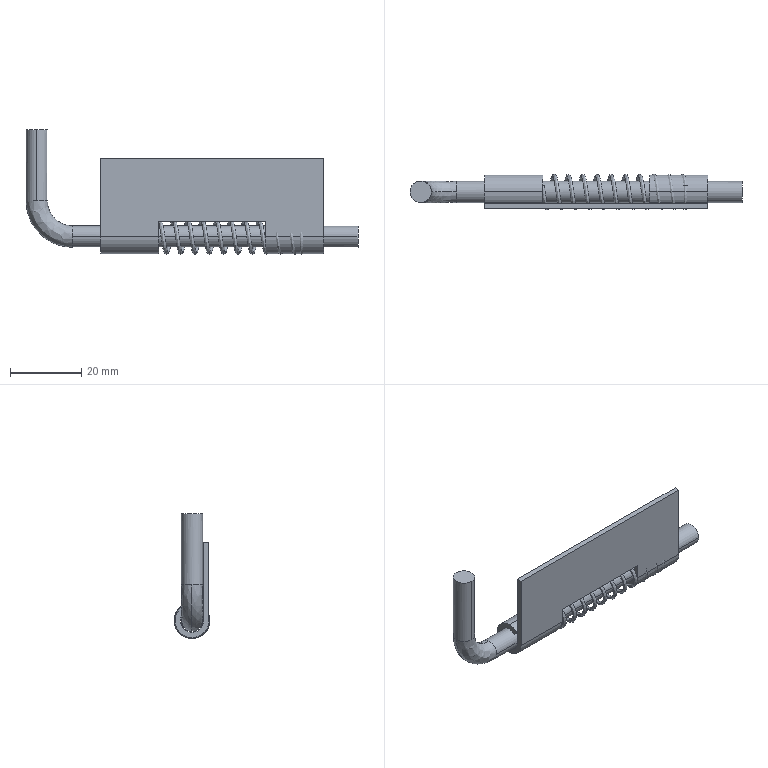Part | STEP file | mirrored door latch (COMPANY_B) | 3 solids | 39 faces | box 93 x 9.976 x 34.988 mm | volume 6427 mm3 | cylinder 18 | plane 15 | spline 6 | commonest cylinder face diameters 6.5 x6 9.5 x6 6 x4 1.5 x2